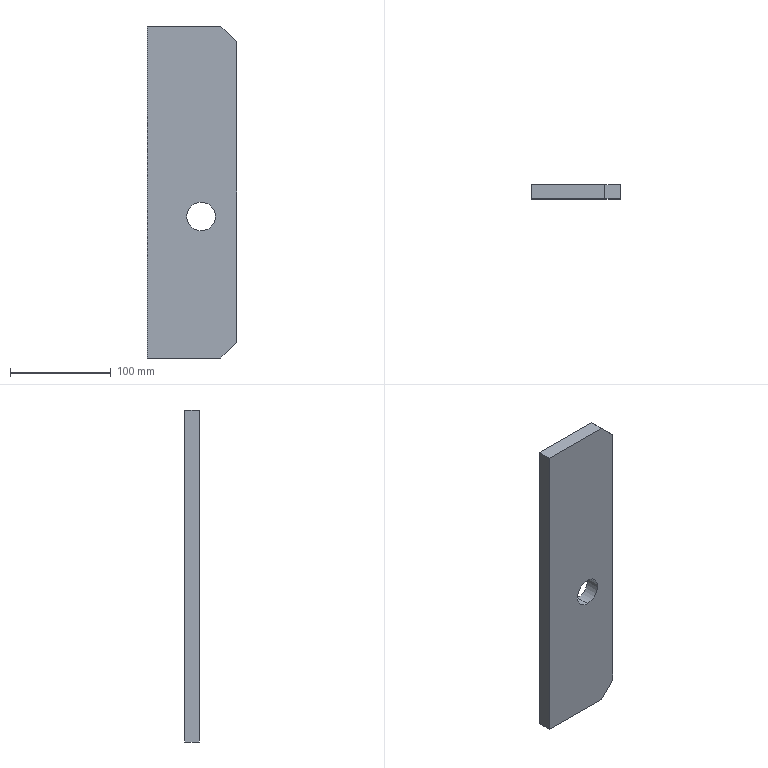Part | SolidWorks | features Extrusion 1 | 1 solid | 10 faces | box 88.9 x 14 x 330.2 mm | volume 398595 mm3 | plane 8 | cylinder 2 | commonest cylinder face diameters 28.448 x2
STEP:
#1=CARTESIAN_POINT('',(0.,7.,-14.224));
#2=VERTEX_POINT('',#1);
#3=CARTESIAN_POINT('',(0.,7.,14.224));
#4=VERTEX_POINT('',#3);
#5=CARTESIAN_POINT('',(0.,7.,0.));
#6=DIRECTION('',(0.,1.,0.));
#7=DIRECTION('',(0.,0.,1.));
#8=AXIS2_PLACEMENT_3D('',#5,#6,#7);
#9=CIRCLE('',#8,14.224);
#10=EDGE_CURVE('',#2,#4,#9,.T.);
#11=ORIENTED_EDGE('',*,*,#10,.T.);
#12=CARTESIAN_POINT('',(0.,-7.,14.224));
#13=VERTEX_POINT('',#12);
#14=CARTESIAN_POINT('',(0.,7.,14.224));
#15=DIRECTION('',(0.,-1.,0.));
#16=VECTOR('',#15,1000.);
#17=LINE('',#14,#16);
#18=EDGE_CURVE('',#4,#13,#17,.T.);
#19=ORIENTED_EDGE('',*,*,#18,.T.);
#20=CARTESIAN_POINT('',(0.,-7.,-14.224));
#21=VERTEX_POINT('',#20);
#22=CARTESIAN_POINT('',(0.,-7.,0.));
#23=DIRECTION('',(0.,1.,0.));
#24=DIRECTION('',(0.,0.,1.));
#25=AXIS2_PLACEMENT_3D('',#22,#23,#24);
#26=CIRCLE('',#25,14.224);
#27=EDGE_CURVE('',#21,#13,#26,.T.);
#28=ORIENTED_EDGE('',*,*,#27,.F.);
#29=CARTESIAN_POINT('',(0.,7.,-14.224));
#30=DIRECTION('',(0.,-1.,0.));
#31=VECTOR('',#30,1000.);
#32=LINE('',#29,#31);
#33=EDGE_CURVE('',#2,#21,#32,.T.);
#34=ORIENTED_EDGE('',*,*,#33,.F.);
#35=EDGE_LOOP('',(#11,#19,#28,#34));
#36=FACE_OUTER_BOUND('',#35,.T.);
#37=CARTESIAN_POINT('',(0.,7.,0.));
#38=DIRECTION('',(0.,-1.,0.));
#39=DIRECTION('',(0.,0.,-1.));
#40=AXIS2_PLACEMENT_3D('',#37,#38,#39);
#41=CYLINDRICAL_SURFACE('',#40,14.224);
#42=ADVANCED_FACE('',(#36),#41,.F.);
#43=CARTESIAN_POINT('',(-53.594,7.,-140.716));
#44=VERTEX_POINT('',#43);
#45=CARTESIAN_POINT('',(-53.594,7.,189.484));
#46=VERTEX_POINT('',#45);
#47=CARTESIAN_POINT('',(-53.594,7.,-140.716));
#48=DIRECTION('',(0.,0.,1.));
#49=VECTOR('',#48,1000.);
#50=LINE('',#47,#49);
#51=EDGE_CURVE('',#44,#46,#50,.T.);
#52=ORIENTED_EDGE('',*,*,#51,.T.);
#53=CARTESIAN_POINT('',(19.556,7.,189.484));
#54=VERTEX_POINT('',#53);
#55=CARTESIAN_POINT('',(-53.594,7.,189.484));
#56=DIRECTION('',(1.,0.,0.));
#57=VECTOR('',#56,1000.);
#58=LINE('',#55,#57);
#59=EDGE_CURVE('',#46,#54,#58,.T.);
#60=ORIENTED_EDGE('',*,*,#59,.T.);
#61=CARTESIAN_POINT('',(35.306,7.,173.734));
#62=VERTEX_POINT('',#61);
#63=CARTESIAN_POINT('',(35.306,7.,173.734));
#64=DIRECTION('',(0.7071,0.,-0.7071));
#65=VECTOR('',#64,1000.);
#66=LINE('',#63,#65);
#67=EDGE_CURVE('',#54,#62,#66,.T.);
#68=ORIENTED_EDGE('',*,*,#67,.T.);
#69=CARTESIAN_POINT('',(35.306,7.,-124.966));
#70=VERTEX_POINT('',#69);
#71=CARTESIAN_POINT('',(35.306,7.,-124.966));
#72=DIRECTION('',(0.,0.,-1.));
#73=VECTOR('',#72,1000.);
#74=LINE('',#71,#73);
#75=EDGE_CURVE('',#62,#70,#74,.T.);
#76=ORIENTED_EDGE('',*,*,#75,.T.);
#77=CARTESIAN_POINT('',(19.556,7.,-140.716));
#78=VERTEX_POINT('',#77);
#79=CARTESIAN_POINT('',(19.556,7.,-140.716));
#80=DIRECTION('',(-0.7071,0.,-0.7071));
#81=VECTOR('',#80,1000.);
#82=LINE('',#79,#81);
#83=EDGE_CURVE('',#70,#78,#82,.T.);
#84=ORIENTED_EDGE('',*,*,#83,.T.);
#85=CARTESIAN_POINT('',(-53.594,7.,-140.716));
#86=DIRECTION('',(-1.,0.,0.));
#87=VECTOR('',#86,1000.);
#88=LINE('',#85,#87);
#89=EDGE_CURVE('',#78,#44,#88,.T.);
#90=ORIENTED_EDGE('',*,*,#89,.T.);
#91=EDGE_LOOP('',(#52,#60,#68,#76,#84,#90));
#92=FACE_OUTER_BOUND('',#91,.T.);
#93=ORIENTED_EDGE('',*,*,#10,.F.);
#94=CARTESIAN_POINT('',(0.,7.,0.));
#95=DIRECTION('',(0.,1.,0.));
#96=DIRECTION('',(0.,0.,1.));
#97=AXIS2_PLACEMENT_3D('',#94,#95,#96);
#98=CIRCLE('',#97,14.224);
#99=EDGE_CURVE('',#4,#2,#98,.T.);
#100=ORIENTED_EDGE('',*,*,#99,.F.);
#101=EDGE_LOOP('',(#93,#100));
#102=FACE_BOUND('',#101,.T.);
#103=CARTESIAN_POINT('',(-53.594,7.,189.484));
#104=DIRECTION('',(0.,1.,0.));
#105=DIRECTION('',(0.,0.,1.));
#106=AXIS2_PLACEMENT_3D('',#103,#104,#105);
#107=PLANE('',#106);
#108=ADVANCED_FACE('',(#92,#102),#107,.T.);
#109=CARTESIAN_POINT('',(-53.594,-7.,-140.716));
#110=VERTEX_POINT('',#109);
#111=CARTESIAN_POINT('',(-53.594,-7.,189.484));
#112=VERTEX_POINT('',#111);
#113=CARTESIAN_POINT('',(-53.594,-7.,-140.716));
#114=DIRECTION('',(0.,0.,1.));
#115=VECTOR('',#114,1000.);
#116=LINE('',#113,#115);
#117=EDGE_CURVE('',#110,#112,#116,.T.);
#118=ORIENTED_EDGE('',*,*,#117,.F.);
#119=CARTESIAN_POINT('',(19.556,-7.,-140.716));
#120=VERTEX_POINT('',#119);
#121=CARTESIAN_POINT('',(-53.594,-7.,-140.716));
#122=DIRECTION('',(-1.,0.,0.));
#123=VECTOR('',#122,1000.);
#124=LINE('',#121,#123);
#125=EDGE_CURVE('',#120,#110,#124,.T.);
#126=ORIENTED_EDGE('',*,*,#125,.F.);
#127=CARTESIAN_POINT('',(35.306,-7.,-124.966));
#128=VERTEX_POINT('',#127);
#129=CARTESIAN_POINT('',(19.556,-7.,-140.716));
#130=DIRECTION('',(-0.7071,0.,-0.7071));
#131=VECTOR('',#130,1000.);
#132=LINE('',#129,#131);
#133=EDGE_CURVE('',#128,#120,#132,.T.);
#134=ORIENTED_EDGE('',*,*,#133,.F.);
#135=CARTESIAN_POINT('',(35.306,-7.,173.734));
#136=VERTEX_POINT('',#135);
#137=CARTESIAN_POINT('',(35.306,-7.,-124.966));
#138=DIRECTION('',(0.,0.,-1.));
#139=VECTOR('',#138,1000.);
#140=LINE('',#137,#139);
#141=EDGE_CURVE('',#136,#128,#140,.T.);
#142=ORIENTED_EDGE('',*,*,#141,.F.);
#143=CARTESIAN_POINT('',(19.556,-7.,189.484));
#144=VERTEX_POINT('',#143);
#145=CARTESIAN_POINT('',(35.306,-7.,173.734));
#146=DIRECTION('',(0.7071,0.,-0.7071));
#147=VECTOR('',#146,1000.);
#148=LINE('',#145,#147);
#149=EDGE_CURVE('',#144,#136,#148,.T.);
#150=ORIENTED_EDGE('',*,*,#149,.F.);
#151=CARTESIAN_POINT('',(-53.594,-7.,189.484));
#152=DIRECTION('',(1.,0.,0.));
#153=VECTOR('',#152,1000.);
#154=LINE('',#151,#153);
#155=EDGE_CURVE('',#112,#144,#154,.T.);
#156=ORIENTED_EDGE('',*,*,#155,.F.);
#157=EDGE_LOOP('',(#118,#126,#134,#142,#150,#156));
#158=FACE_OUTER_BOUND('',#157,.T.);
#159=ORIENTED_EDGE('',*,*,#27,.T.);
#160=CARTESIAN_POINT('',(0.,-7.,0.));
#161=DIRECTION('',(0.,1.,0.));
#162=DIRECTION('',(0.,0.,1.));
#163=AXIS2_PLACEMENT_3D('',#160,#161,#162);
#164=CIRCLE('',#163,14.224);
#165=EDGE_CURVE('',#13,#21,#164,.T.);
#166=ORIENTED_EDGE('',*,*,#165,.T.);
#167=EDGE_LOOP('',(#159,#166));
#168=FACE_BOUND('',#167,.T.);
#169=CARTESIAN_POINT('',(-53.594,-7.,189.484));
#170=DIRECTION('',(0.,1.,0.));
#171=DIRECTION('',(0.,0.,1.));
#172=AXIS2_PLACEMENT_3D('',#169,#170,#171);
#173=PLANE('',#172);
#174=ADVANCED_FACE('',(#158,#168),#173,.F.);
#175=ORIENTED_EDGE('',*,*,#117,.T.);
#176=CARTESIAN_POINT('',(-53.594,7.,189.484));
#177=DIRECTION('',(0.,-1.,0.));
#178=VECTOR('',#177,1000.);
#179=LINE('',#176,#178);
#180=EDGE_CURVE('',#46,#112,#179,.T.);
#181=ORIENTED_EDGE('',*,*,#180,.F.);
#182=ORIENTED_EDGE('',*,*,#51,.F.);
#183=CARTESIAN_POINT('',(-53.594,7.,-140.716));
#184=DIRECTION('',(0.,-1.,0.));
#185=VECTOR('',#184,1000.);
#186=LINE('',#183,#185);
#187=EDGE_CURVE('',#44,#110,#186,.T.);
#188=ORIENTED_EDGE('',*,*,#187,.T.);
#189=EDGE_LOOP('',(#175,#181,#182,#188));
#190=FACE_OUTER_BOUND('',#189,.T.);
#191=CARTESIAN_POINT('',(-53.594,7.,-140.716));
#192=DIRECTION('',(1.,0.,0.));
#193=DIRECTION('',(0.,0.,-1.));
#194=AXIS2_PLACEMENT_3D('',#191,#192,#193);
#195=PLANE('',#194);
#196=ADVANCED_FACE('',(#190),#195,.F.);
#197=ORIENTED_EDGE('',*,*,#155,.T.);
#198=CARTESIAN_POINT('',(19.556,7.,189.484));
#199=DIRECTION('',(0.,-1.,0.));
#200=VECTOR('',#199,1000.);
#201=LINE('',#198,#200);
#202=EDGE_CURVE('',#54,#144,#201,.T.);
#203=ORIENTED_EDGE('',*,*,#202,.F.);
#204=ORIENTED_EDGE('',*,*,#59,.F.);
#205=ORIENTED_EDGE('',*,*,#180,.T.);
#206=EDGE_LOOP('',(#197,#203,#204,#205));
#207=FACE_OUTER_BOUND('',#206,.T.);
#208=CARTESIAN_POINT('',(-53.594,7.,189.484));
#209=DIRECTION('',(0.,0.,-1.));
#210=DIRECTION('',(-1.,0.,0.));
#211=AXIS2_PLACEMENT_3D('',#208,#209,#210);
#212=PLANE('',#211);
#213=ADVANCED_FACE('',(#207),#212,.F.);
#214=ORIENTED_EDGE('',*,*,#149,.T.);
#215=CARTESIAN_POINT('',(35.306,7.,173.734));
#216=DIRECTION('',(0.,-1.,0.));
#217=VECTOR('',#216,1000.);
#218=LINE('',#215,#217);
#219=EDGE_CURVE('',#62,#136,#218,.T.);
#220=ORIENTED_EDGE('',*,*,#219,.F.);
#221=ORIENTED_EDGE('',*,*,#67,.F.);
#222=ORIENTED_EDGE('',*,*,#202,.T.);
#223=EDGE_LOOP('',(#214,#220,#221,#222));
#224=FACE_OUTER_BOUND('',#223,.T.);
#225=CARTESIAN_POINT('',(35.306,7.,173.734));
#226=DIRECTION('',(-0.7071,0.,-0.7071));
#227=DIRECTION('',(-0.7071,0.,0.7071));
#228=AXIS2_PLACEMENT_3D('',#225,#226,#227);
#229=PLANE('',#228);
#230=ADVANCED_FACE('',(#224),#229,.F.);
#231=ORIENTED_EDGE('',*,*,#141,.T.);
#232=CARTESIAN_POINT('',(35.306,7.,-124.966));
#233=DIRECTION('',(0.,-1.,0.));
#234=VECTOR('',#233,1000.);
#235=LINE('',#232,#234);
#236=EDGE_CURVE('',#70,#128,#235,.T.);
#237=ORIENTED_EDGE('',*,*,#236,.F.);
#238=ORIENTED_EDGE('',*,*,#75,.F.);
#239=ORIENTED_EDGE('',*,*,#219,.T.);
#240=EDGE_LOOP('',(#231,#237,#238,#239));
#241=FACE_OUTER_BOUND('',#240,.T.);
#242=CARTESIAN_POINT('',(35.306,7.,-124.966));
#243=DIRECTION('',(-1.,0.,0.));
#244=DIRECTION('',(0.,0.,1.));
#245=AXIS2_PLACEMENT_3D('',#242,#243,#244);
#246=PLANE('',#245);
#247=ADVANCED_FACE('',(#241),#246,.F.);
#248=ORIENTED_EDGE('',*,*,#133,.T.);
#249=CARTESIAN_POINT('',(19.556,7.,-140.716));
#250=DIRECTION('',(0.,-1.,0.));
#251=VECTOR('',#250,1000.);
#252=LINE('',#249,#251);
#253=EDGE_CURVE('',#78,#120,#252,.T.);
#254=ORIENTED_EDGE('',*,*,#253,.F.);
#255=ORIENTED_EDGE('',*,*,#83,.F.);
#256=ORIENTED_EDGE('',*,*,#236,.T.);
#257=EDGE_LOOP('',(#248,#254,#255,#256));
#258=FACE_OUTER_BOUND('',#257,.T.);
#259=CARTESIAN_POINT('',(19.556,7.,-140.716));
#260=DIRECTION('',(-0.7071,0.,0.7071));
#261=DIRECTION('',(0.7071,0.,0.7071));
#262=AXIS2_PLACEMENT_3D('',#259,#260,#261);
#263=PLANE('',#262);
#264=ADVANCED_FACE('',(#258),#263,.F.);
#265=ORIENTED_EDGE('',*,*,#125,.T.);
#266=ORIENTED_EDGE('',*,*,#187,.F.);
#267=ORIENTED_EDGE('',*,*,#89,.F.);
#268=ORIENTED_EDGE('',*,*,#253,.T.);
#269=EDGE_LOOP('',(#265,#266,#267,#268));
#270=FACE_OUTER_BOUND('',#269,.T.);
#271=CARTESIAN_POINT('',(-53.594,7.,-140.716));
#272=DIRECTION('',(0.,0.,1.));
#273=DIRECTION('',(1.,0.,0.));
#274=AXIS2_PLACEMENT_3D('',#271,#272,#273);
#275=PLANE('',#274);
#276=ADVANCED_FACE('',(#270),#275,.F.);
#277=ORIENTED_EDGE('',*,*,#18,.F.);
#278=ORIENTED_EDGE('',*,*,#99,.T.);
#279=ORIENTED_EDGE('',*,*,#33,.T.);
#280=ORIENTED_EDGE('',*,*,#165,.F.);
#281=EDGE_LOOP('',(#277,#278,#279,#280));
#282=FACE_OUTER_BOUND('',#281,.T.);
#283=CARTESIAN_POINT('',(0.,7.,0.));
#284=DIRECTION('',(0.,-1.,0.));
#285=DIRECTION('',(0.,0.,-1.));
#286=AXIS2_PLACEMENT_3D('',#283,#284,#285);
#287=CYLINDRICAL_SURFACE('',#286,14.224);
#288=ADVANCED_FACE('',(#282),#287,.F.);
#289=CLOSED_SHELL('',(#42,#108,#174,#196,#213,#230,#247,#264,#276,#288));
#290=MANIFOLD_SOLID_BREP('',#289);
#291=CARTESIAN_POINT('',(0.,0.,0.));
#292=DIRECTION('',(0.,0.,1.));
#293=DIRECTION('',(1.,0.,0.));
#294=AXIS2_PLACEMENT_3D('',#291,#292,#293);
#295=(LENGTH_UNIT()NAMED_UNIT(*)SI_UNIT(.MILLI.,.METRE.));
#296=UNCERTAINTY_MEASURE_WITH_UNIT(LENGTH_MEASURE(0.00001),#295,'','');
#297=(NAMED_UNIT(*)PLANE_ANGLE_UNIT()SI_UNIT($,.RADIAN.));
#298=(NAMED_UNIT(*)SI_UNIT($,.STERADIAN.)SOLID_ANGLE_UNIT());
#299=(GEOMETRIC_REPRESENTATION_CONTEXT(3)GLOBAL_UNCERTAINTY_ASSIGNED_CONTEXT((#296))GLOBAL_UNIT_ASSIGNED_CONTEXT((#295,#297,#298))REPRESENTATION_CONTEXT('',''));
#300=ADVANCED_BREP_SHAPE_REPRESENTATION('',(#290,#294),#299);